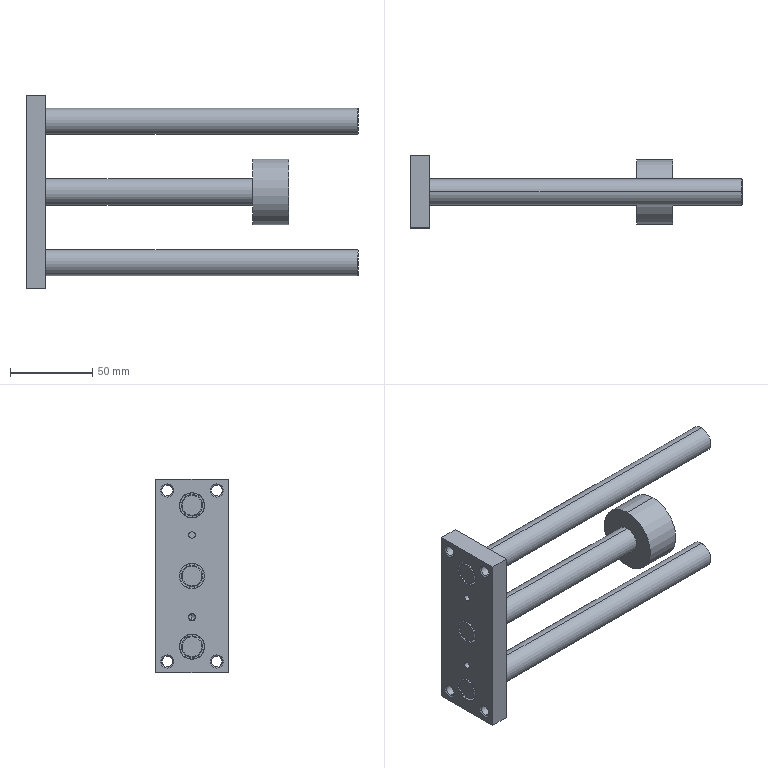Part | NX | features BREP 1 | 1 solid | 90 faces | box 202 x 44 x 118 mm | volume 188629 mm3 | cylinder 35 | cone 28 | plane 21 | torus 6 | commonest cylinder face diameters 6.647 x8 4 x7 13 x6 15 x6 16 x6 39.6 x2